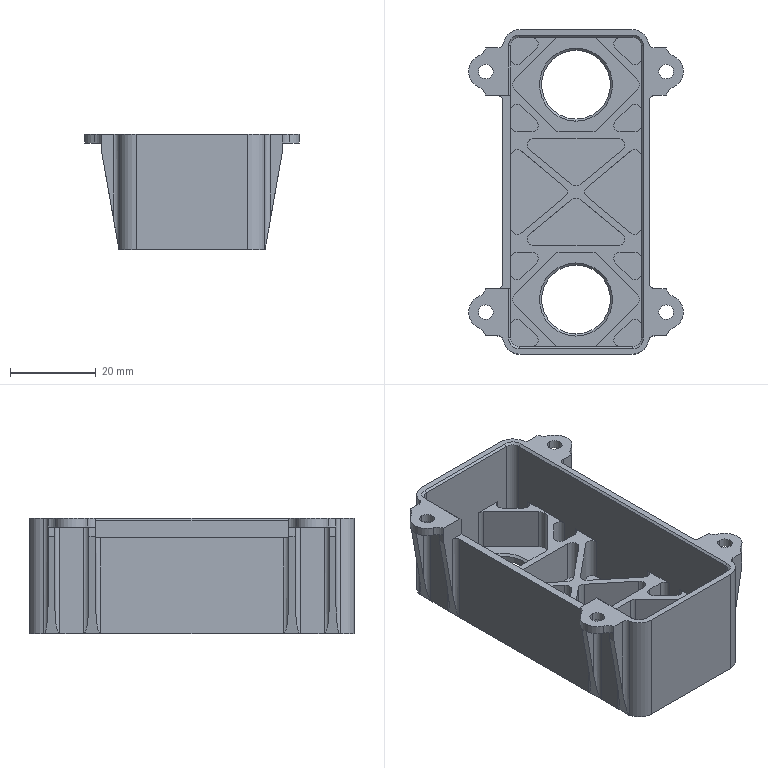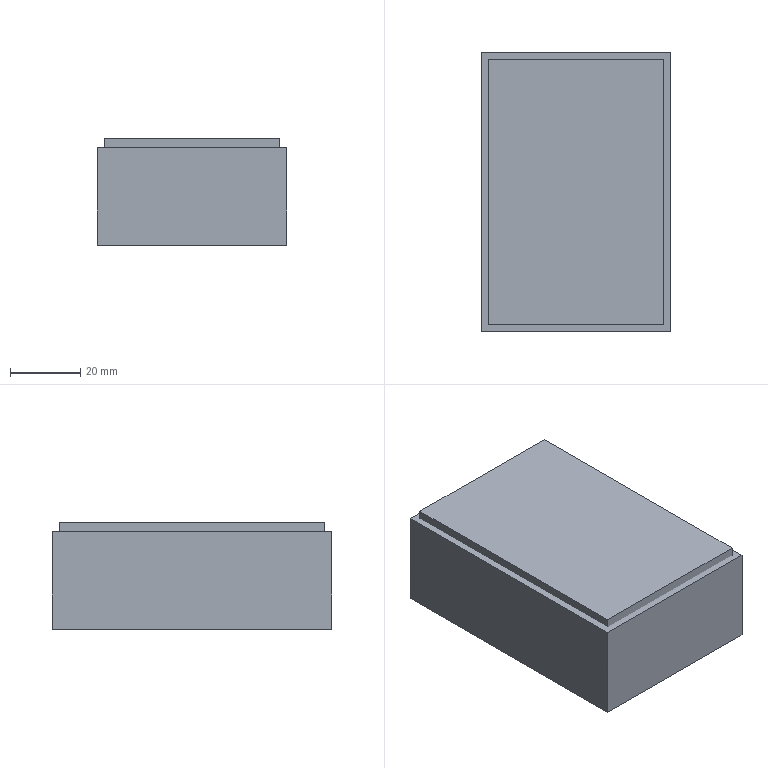CAM job | NX | 3-axis milling, drilling | part box 50 x 75.58 x 26.8 mm | stock box 54 x 79.58 x 30.3 mm
Tools:
number,name,description,diameter,corner_radius,flute_length,length,flutes
19,D80,Milling Tool-5 Parameters,80.0,0.0,50.0,75.0,2
15,D10,Milling Tool-5 Parameters,10.0,0.0,50.0,75.0,2
14,D10JING,Milling Tool-5 Parameters,10.0,0.0,50.0,75.0,2
12,D6,Milling Tool-5 Parameters,6.0,0.0,50.0,75.0,2
16,D6R0.5,Milling Tool-5 Parameters,6.0,0.5,50.0,75.0,2
17,D3,Milling Tool-5 Parameters,3.0,0.0,50.0,75.0,2
1,D6A45,Milling Tool-5 Parameters,6.0,0.0,50.0,75.0,2
11,D4,Milling Tool-5 Parameters,4.0,0.0,50.0,75.0,2
3,3.4ZT,Drilling Tool,3.4,0.0,35.0,50.0,2
Operations:
program,operation,operation_type,tool,method,geometry_group,spindle_rpm,surface_speed,feed_per_tooth,feed_cut,feed_plunge,cut_length_mm,path_length_mm,cut_time_min,machine_time_min
1,FLOOR_WALL_COPY,VolumeBased25DMillingOperation,D80,METHOD,A,6500.0,1633.0,0.1154,1500.0,100.0,175.58,229.58,0.1171,0.1225
1,ZLEVEL_PROFILE_COPY,ZLevelMilling,D10,METHOD,A,9500.0,298.0,0.1684,3200.0,1000.0,7345.529,7429.329,2.328,2.337
1,ZLEVEL_PROFILE,ZLevelMilling,D10,METHOD,A,9500.0,298.0,0.1684,3200.0,1000.0,7340.784,7424.584,2.327,2.335
1,HOLE_MILLING,CylinderMilling,D10,METHOD,A,9500.0,298.0,0.1158,2200.0,100.0,166.98,338.98,0.0759,0.0931
1,ZLEVEL_PROFILE_COPY_1_COPY_COPY_1_COPY_COPY_1_COPY,ZLevelMilling,D10JING,METHOD,A,9500.0,298.0,0.0632,1200.0,1000.0,44.824,224.244,0.0379,0.0559
1,ZLEVEL_PROFILE_COPY_1_COPY_COPY_1_COPY_COPY_1,ZLevelMilling,D10JING,METHOD,A,9500.0,298.0,0.0632,1200.0,1000.0,540.075,737.651,0.4506,0.4704
1,ZLEVEL_PROFILE_COPY_1,ZLevelMilling,D6,METHOD,A,9500.0,179.0,0.0789,1500.0,1000.0,4440.601,12340.683,3.339,4.129
1,ZLEVEL_PROFILE_1,ZLevelMilling,D6R0.5,METHOD,A,9500.0,119.0,0.1842,3500.0,100.0,5747.86,6611.542,1.642,1.729
1,ZLEVEL_PROFILE_COPY_1_COPY,ZLevelMilling,D3,METHOD,A,8000.0,75.0,0.05,800.0,1000.0,8630.65,15062.554,10.382,11.025
1,PLANAR_MILL_COPY_COPY_COPY_COPY_COPY_COPY_1_COPY_1,PlanarMilling,D6A45,METHOD,A,9500.0,179.0,0.0658,1250.0,100.0,323.103,572.714,0.2585,0.2834
2,FLOOR_WALL_COPY_COPY,VolumeBased25DMillingOperation,D80,METHOD,B,6500.0,1633.0,0.1154,1500.0,100.0,686.32,1388.561,0.4575,0.5278
2,DRILLING_COPY_1,Operation,D6A45,METHOD,B,5000.0,94.0,0.035,350.0,0.0,16.4,298.009,0.0469,0.075
2,DRILLING_COPY_1_COPY_1_1_COPY_1,Operation,3.4ZT,METHOD,B,2000.0,34.0,0.05,200.0,0.0,30.086,269.466,0.1504,0.1744
2,FLOOR_WALL,VolumeBased25DMillingOperation,D10,METHOD,B,9500.0,0.0,0.0,2000.0,1000.0,1718.15,1841.193,0.874,0.8863
2,CAVITY_MILL_COPY_1,CavityMilling,D10,METHOD,B,9500.0,298.0,0.1316,2500.0,1000.0,8887.138,9768.495,5.145,5.233
2,CAVITY_MILL_COPY_COPY,CavityMilling,D4,METHOD,B,9500.0,119.0,0.0737,1400.0,1000.0,17222.963,23523.732,14.437,15.067
2,FLOOR_WALL_COPY_1,VolumeBased25DMillingOperation,D4,METHOD,B,9500.0,179.0,0.0579,1100.0,100.0,2163.892,4871.777,1.967,2.238
2,CAVITY_MILL_COPY_COPY_COPY,CavityMilling,D3,METHOD,B,8500.0,80.0,0.0471,800.0,1000.0,15024.214,20201.331,17.59,18.108
2,PLANAR_MILL_COPY_COPY_COPY_COPY_COPY_COPY_1_COPY_1_COPY,PlanarMilling,D6A45,METHOD,B,9500.0,179.0,0.0658,1250.0,100.0,418.405,855.611,0.3347,0.3784
2,PLANAR_MILL_COPY_COPY_COPY_COPY_COPY_COPY_1_COPY_1_COPY_COPY_1,PlanarMilling,D6A45,METHOD,B,9500.0,179.0,0.0658,1250.0,100.0,390.384,2022.666,0.3123,0.4755
2,PLANAR_MILL_COPY_COPY_COPY_COPY_COPY_COPY_1_COPY_1_COPY_COPY,PlanarMilling,D6A45,METHOD,B,9500.0,179.0,0.0658,1250.0,100.0,104.437,371.667,0.0835,0.1103
PROGRAM,FLOOR_WALL_COPY_1_COPY,VolumeBased25DMillingOperation,D4,METHOD,B,9500.0,179.0,0.0579,1100.0,100.0,567.807,2519.862,0.5162,0.7114